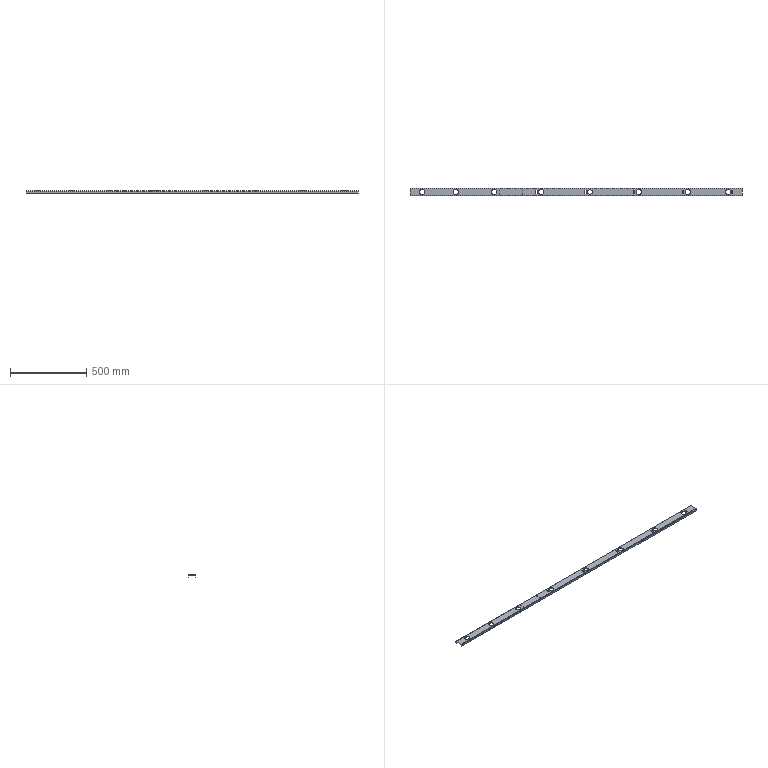Part | NX | features solid 2 | 1 solid | 60 faces | box 2173 x 52 x 16.5 mm | volume 311174 mm3 | plane 32 | cylinder 28 | commonest cylinder face diameters 35 x14 3 x8 4 x2 8 x2 30 x2